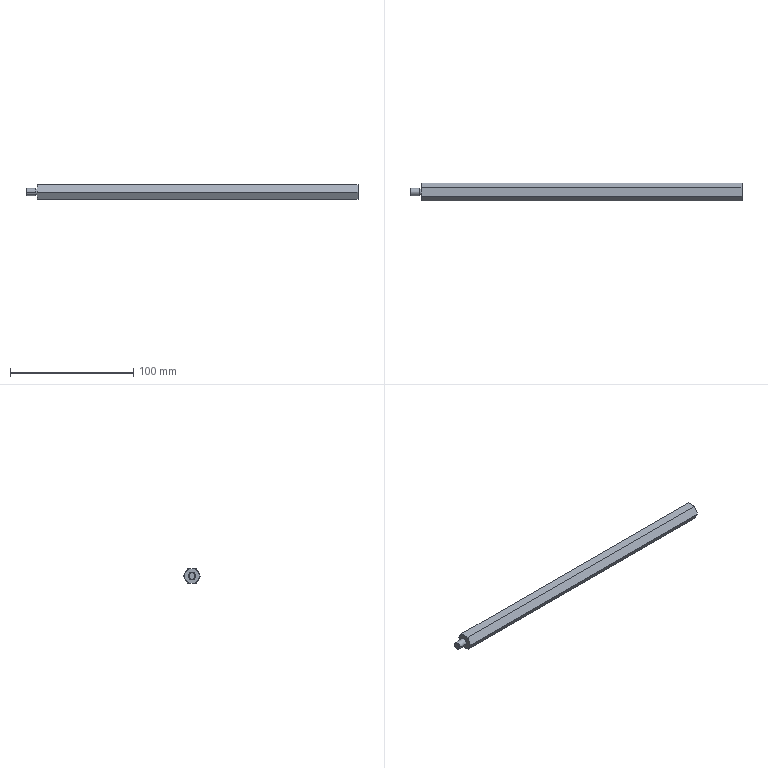Part | NX | 1 solid | 31 faces | box 269 x 13.856 x 12 mm | volume 32453 mm3 | cone 13 | plane 10 | cylinder 8 | commonest cylinder face diameters 4.2 x4 4.917 x2 6 x2
STEP:
#1=CARTESIAN_POINT('',(0.,5.196,-3.));
#2=VERTEX_POINT('',#1);
#3=CARTESIAN_POINT('',(0.5359,6.928,0.));
#4=VERTEX_POINT('',#3);
#5=CARTESIAN_POINT('',(0.,5.196,-3.));
#6=CARTESIAN_POINT('',(0.,5.754,-2.033));
#7=CARTESIAN_POINT('',(0.1777,6.308,-1.074));
#8=CARTESIAN_POINT('',(0.5359,6.928,0.));
#9=B_SPLINE_CURVE_WITH_KNOTS('',3,(#5,#6,#7,#8),.UNSPECIFIED.,.F.,.F.,(4,4),(0.,1.),.UNSPECIFIED.);
#10=EDGE_CURVE('',#2,#4,#9,.T.);
#11=ORIENTED_EDGE('',*,*,#10,.F.);
#12=CARTESIAN_POINT('',(0.,5.196,3.));
#13=VERTEX_POINT('',#12);
#14=CARTESIAN_POINT('',(0.,0.,0.));
#15=DIRECTION('',(1.,0.,0.));
#16=DIRECTION('',(0.,0.866,-0.5));
#17=AXIS2_PLACEMENT_3D('',#14,#15,#16);
#18=CIRCLE('',#17,6.);
#19=EDGE_CURVE('',#2,#13,#18,.T.);
#20=ORIENTED_EDGE('',*,*,#19,.T.);
#21=CARTESIAN_POINT('',(0.5359,6.928,0.));
#22=CARTESIAN_POINT('',(0.1786,6.309,1.072));
#23=CARTESIAN_POINT('',(0.,5.732,2.072));
#24=CARTESIAN_POINT('',(0.,5.196,3.));
#25=B_SPLINE_CURVE_WITH_KNOTS('',3,(#21,#22,#23,#24),.UNSPECIFIED.,.F.,.F.,(4,4),(0.,1.),.UNSPECIFIED.);
#26=EDGE_CURVE('',#13,#4,#25,.F.);
#27=ORIENTED_EDGE('',*,*,#26,.T.);
#28=EDGE_LOOP('',(#11,#20,#27));
#29=FACE_BOUND('',#28,.T.);
#30=CARTESIAN_POINT('',(0.2679,0.,0.));
#31=DIRECTION('',(1.,0.,0.));
#32=DIRECTION('',(0.,-1.,0.));
#33=AXIS2_PLACEMENT_3D('',#30,#31,#32);
#34=CONICAL_SURFACE('',#33,6.464,1.047);
#35=ADVANCED_FACE('',(#29),#34,.T.);
#36=CARTESIAN_POINT('',(-8.459,-3.,0.));
#37=VERTEX_POINT('',#36);
#38=CARTESIAN_POINT('',(-8.459,3.,0.));
#39=VERTEX_POINT('',#38);
#40=CARTESIAN_POINT('',(-8.459,0.,0.));
#41=DIRECTION('',(1.,0.,0.));
#42=DIRECTION('',(0.,1.,0.));
#43=AXIS2_PLACEMENT_3D('',#40,#41,#42);
#44=CIRCLE('',#43,3.);
#45=EDGE_CURVE('',#37,#39,#44,.T.);
#46=ORIENTED_EDGE('',*,*,#45,.F.);
#47=CARTESIAN_POINT('',(-9.,-2.459,0.));
#48=VERTEX_POINT('',#47);
#49=CARTESIAN_POINT('',(-8.729,-2.729,0.));
#50=DIRECTION('',(0.7071,-0.7071,0.));
#51=VECTOR('',#50,1000.);
#52=LINE('',#49,#51);
#53=EDGE_CURVE('',#37,#48,#52,.F.);
#54=ORIENTED_EDGE('',*,*,#53,.T.);
#55=CARTESIAN_POINT('',(-9.,2.459,0.));
#56=VERTEX_POINT('',#55);
#57=CARTESIAN_POINT('',(-9.,0.,0.));
#58=DIRECTION('',(1.,0.,0.));
#59=DIRECTION('',(0.,1.,0.));
#60=AXIS2_PLACEMENT_3D('',#57,#58,#59);
#61=CIRCLE('',#60,2.458);
#62=EDGE_CURVE('',#48,#56,#61,.T.);
#63=ORIENTED_EDGE('',*,*,#62,.T.);
#64=CARTESIAN_POINT('',(-8.729,2.729,0.));
#65=DIRECTION('',(0.7071,0.7071,0.));
#66=VECTOR('',#65,1000.);
#67=LINE('',#64,#66);
#68=EDGE_CURVE('',#39,#56,#67,.F.);
#69=ORIENTED_EDGE('',*,*,#68,.F.);
#70=EDGE_LOOP('',(#46,#54,#63,#69));
#71=FACE_BOUND('',#70,.T.);
#72=CARTESIAN_POINT('',(-8.729,0.,0.));
#73=DIRECTION('',(1.,0.,0.));
#74=DIRECTION('',(0.,-1.,0.));
#75=AXIS2_PLACEMENT_3D('',#72,#73,#74);
#76=CONICAL_SURFACE('',#75,2.729,0.7854);
#77=ADVANCED_FACE('',(#71),#76,.T.);
#78=CARTESIAN_POINT('',(260.,3.464,6.));
#79=VERTEX_POINT('',#78);
#80=CARTESIAN_POINT('',(260.,6.928,0.));
#81=VERTEX_POINT('',#80);
#82=CARTESIAN_POINT('',(260.,6.928,0.));
#83=DIRECTION('',(0.,0.5,-0.866));
#84=VECTOR('',#83,1000.);
#85=LINE('',#82,#84);
#86=EDGE_CURVE('',#79,#81,#85,.T.);
#87=ORIENTED_EDGE('',*,*,#86,.T.);
#88=CARTESIAN_POINT('',(260.,6.928,0.));
#89=DIRECTION('',(-1.,0.,0.));
#90=VECTOR('',#89,1000.);
#91=LINE('',#88,#90);
#92=EDGE_CURVE('',#81,#4,#91,.T.);
#93=ORIENTED_EDGE('',*,*,#92,.T.);
#94=ORIENTED_EDGE('',*,*,#26,.F.);
#95=CARTESIAN_POINT('',(0.5359,3.464,6.));
#96=VERTEX_POINT('',#95);
#97=CARTESIAN_POINT('',(0.,5.196,3.));
#98=CARTESIAN_POINT('',(0.,4.66,3.928));
#99=CARTESIAN_POINT('',(0.1786,4.083,4.928));
#100=CARTESIAN_POINT('',(0.5359,3.464,6.));
#101=B_SPLINE_CURVE_WITH_KNOTS('',3,(#97,#98,#99,#100),.UNSPECIFIED.,.F.,.F.,(4,4),(0.,1.),.UNSPECIFIED.);
#102=EDGE_CURVE('',#96,#13,#101,.F.);
#103=ORIENTED_EDGE('',*,*,#102,.F.);
#104=CARTESIAN_POINT('',(0.5359,3.464,6.));
#105=DIRECTION('',(1.,0.,0.));
#106=VECTOR('',#105,1000.);
#107=LINE('',#104,#106);
#108=EDGE_CURVE('',#96,#79,#107,.T.);
#109=ORIENTED_EDGE('',*,*,#108,.T.);
#110=EDGE_LOOP('',(#87,#93,#94,#103,#109));
#111=FACE_BOUND('',#110,.T.);
#112=CARTESIAN_POINT('',(155.,5.196,3.));
#113=DIRECTION('',(0.,-0.866,-0.5));
#114=DIRECTION('',(0.,0.5,-0.866));
#115=AXIS2_PLACEMENT_3D('',#112,#113,#114);
#116=PLANE('',#115);
#117=ADVANCED_FACE('',(#111),#116,.F.);
#118=CARTESIAN_POINT('',(260.,3.464,-6.));
#119=VERTEX_POINT('',#118);
#120=CARTESIAN_POINT('',(260.,-3.464,-6.));
#121=VERTEX_POINT('',#120);
#122=CARTESIAN_POINT('',(260.,0.,-6.));
#123=DIRECTION('',(0.,-1.,0.));
#124=VECTOR('',#123,1000.);
#125=LINE('',#122,#124);
#126=EDGE_CURVE('',#119,#121,#125,.T.);
#127=ORIENTED_EDGE('',*,*,#126,.F.);
#128=CARTESIAN_POINT('',(260.,6.928,0.));
#129=DIRECTION('',(0.,-0.5,-0.866));
#130=VECTOR('',#129,1000.);
#131=LINE('',#128,#130);
#132=EDGE_CURVE('',#81,#119,#131,.T.);
#133=ORIENTED_EDGE('',*,*,#132,.F.);
#134=ORIENTED_EDGE('',*,*,#86,.F.);
#135=CARTESIAN_POINT('',(260.,-3.464,6.));
#136=VERTEX_POINT('',#135);
#137=CARTESIAN_POINT('',(260.,0.,6.));
#138=DIRECTION('',(0.,1.,0.));
#139=VECTOR('',#138,1000.);
#140=LINE('',#137,#139);
#141=EDGE_CURVE('',#136,#79,#140,.T.);
#142=ORIENTED_EDGE('',*,*,#141,.F.);
#143=CARTESIAN_POINT('',(260.,-6.928,0.));
#144=VERTEX_POINT('',#143);
#145=CARTESIAN_POINT('',(260.,-6.928,0.));
#146=DIRECTION('',(0.,0.5,0.866));
#147=VECTOR('',#146,1000.);
#148=LINE('',#145,#147);
#149=EDGE_CURVE('',#144,#136,#148,.T.);
#150=ORIENTED_EDGE('',*,*,#149,.F.);
#151=CARTESIAN_POINT('',(260.,-6.928,0.));
#152=DIRECTION('',(0.,-0.5,0.866));
#153=VECTOR('',#152,1000.);
#154=LINE('',#151,#153);
#155=EDGE_CURVE('',#121,#144,#154,.T.);
#156=ORIENTED_EDGE('',*,*,#155,.F.);
#157=EDGE_LOOP('',(#127,#133,#134,#142,#150,#156));
#158=FACE_BOUND('',#157,.T.);
#159=CARTESIAN_POINT('',(260.,2.86,0.));
#160=VERTEX_POINT('',#159);
#161=CARTESIAN_POINT('',(260.,-2.86,0.));
#162=VERTEX_POINT('',#161);
#163=CARTESIAN_POINT('',(260.,0.,0.));
#164=DIRECTION('',(1.,0.,0.));
#165=DIRECTION('',(0.,-1.,0.));
#166=AXIS2_PLACEMENT_3D('',#163,#164,#165);
#167=CIRCLE('',#166,2.86);
#168=EDGE_CURVE('',#160,#162,#167,.T.);
#169=ORIENTED_EDGE('',*,*,#168,.F.);
#170=CARTESIAN_POINT('',(260.,0.,0.));
#171=DIRECTION('',(1.,0.,0.));
#172=DIRECTION('',(0.,-1.,0.));
#173=AXIS2_PLACEMENT_3D('',#170,#171,#172);
#174=CIRCLE('',#173,2.86);
#175=EDGE_CURVE('',#162,#160,#174,.T.);
#176=ORIENTED_EDGE('',*,*,#175,.F.);
#177=EDGE_LOOP('',(#169,#176));
#178=FACE_BOUND('',#177,.T.);
#179=CARTESIAN_POINT('',(260.,-6.371,11.678));
#180=DIRECTION('',(-1.,0.,0.));
#181=DIRECTION('',(0.,0.,1.));
#182=AXIS2_PLACEMENT_3D('',#179,#180,#181);
#183=PLANE('',#182);
#184=ADVANCED_FACE('',(#158,#178),#183,.F.);
#185=ORIENTED_EDGE('',*,*,#126,.T.);
#186=CARTESIAN_POINT('',(0.5359,-3.464,-6.));
#187=VERTEX_POINT('',#186);
#188=CARTESIAN_POINT('',(260.,-3.464,-6.));
#189=DIRECTION('',(-1.,0.,0.));
#190=VECTOR('',#189,1000.);
#191=LINE('',#188,#190);
#192=EDGE_CURVE('',#121,#187,#191,.T.);
#193=ORIENTED_EDGE('',*,*,#192,.T.);
#194=CARTESIAN_POINT('',(0.,0.,-6.));
#195=VERTEX_POINT('',#194);
#196=CARTESIAN_POINT('',(0.5359,-3.464,-6.));
#197=CARTESIAN_POINT('',(0.1786,-2.226,-6.));
#198=CARTESIAN_POINT('',(0.,-1.072,-6.));
#199=CARTESIAN_POINT('',(0.,0.,-6.));
#200=B_SPLINE_CURVE_WITH_KNOTS('',3,(#196,#197,#198,#199),.UNSPECIFIED.,.F.,.F.,(4,4),(0.,1.),.UNSPECIFIED.);
#201=EDGE_CURVE('',#195,#187,#200,.F.);
#202=ORIENTED_EDGE('',*,*,#201,.F.);
#203=CARTESIAN_POINT('',(0.5359,3.464,-6.));
#204=VERTEX_POINT('',#203);
#205=CARTESIAN_POINT('',(0.,0.,-6.));
#206=CARTESIAN_POINT('',(0.,1.072,-6.));
#207=CARTESIAN_POINT('',(0.1786,2.226,-6.));
#208=CARTESIAN_POINT('',(0.5359,3.464,-6.));
#209=B_SPLINE_CURVE_WITH_KNOTS('',3,(#205,#206,#207,#208),.UNSPECIFIED.,.F.,.F.,(4,4),(0.,1.),.UNSPECIFIED.);
#210=EDGE_CURVE('',#204,#195,#209,.F.);
#211=ORIENTED_EDGE('',*,*,#210,.F.);
#212=CARTESIAN_POINT('',(0.5359,3.464,-6.));
#213=DIRECTION('',(1.,0.,0.));
#214=VECTOR('',#213,1000.);
#215=LINE('',#212,#214);
#216=EDGE_CURVE('',#204,#119,#215,.T.);
#217=ORIENTED_EDGE('',*,*,#216,.T.);
#218=EDGE_LOOP('',(#185,#193,#202,#211,#217));
#219=FACE_BOUND('',#218,.T.);
#220=CARTESIAN_POINT('',(155.,0.,-6.));
#221=DIRECTION('',(0.,0.,1.));
#222=DIRECTION('',(1.,0.,0.));
#223=AXIS2_PLACEMENT_3D('',#220,#221,#222);
#224=PLANE('',#223);
#225=ADVANCED_FACE('',(#219),#224,.F.);
#226=ORIENTED_EDGE('',*,*,#132,.T.);
#227=ORIENTED_EDGE('',*,*,#216,.F.);
#228=CARTESIAN_POINT('',(0.5359,3.464,-6.));
#229=CARTESIAN_POINT('',(0.1786,4.083,-4.928));
#230=CARTESIAN_POINT('',(0.,4.66,-3.928));
#231=CARTESIAN_POINT('',(0.,5.196,-3.));
#232=B_SPLINE_CURVE_WITH_KNOTS('',3,(#228,#229,#230,#231),.UNSPECIFIED.,.F.,.F.,(4,4),(0.,1.),.UNSPECIFIED.);
#233=EDGE_CURVE('',#2,#204,#232,.F.);
#234=ORIENTED_EDGE('',*,*,#233,.F.);
#235=ORIENTED_EDGE('',*,*,#10,.T.);
#236=ORIENTED_EDGE('',*,*,#92,.F.);
#237=EDGE_LOOP('',(#226,#227,#234,#235,#236));
#238=FACE_BOUND('',#237,.T.);
#239=CARTESIAN_POINT('',(155.,5.196,-3.));
#240=DIRECTION('',(0.,-0.866,0.5));
#241=DIRECTION('',(-1.,0.,0.));
#242=AXIS2_PLACEMENT_3D('',#239,#240,#241);
#243=PLANE('',#242);
#244=ADVANCED_FACE('',(#238),#243,.F.);
#245=ORIENTED_EDGE('',*,*,#210,.T.);
#246=CARTESIAN_POINT('',(0.,0.,0.));
#247=DIRECTION('',(1.,0.,0.));
#248=DIRECTION('',(0.,0.,-1.));
#249=AXIS2_PLACEMENT_3D('',#246,#247,#248);
#250=CIRCLE('',#249,6.);
#251=EDGE_CURVE('',#195,#2,#250,.T.);
#252=ORIENTED_EDGE('',*,*,#251,.T.);
#253=ORIENTED_EDGE('',*,*,#233,.T.);
#254=EDGE_LOOP('',(#245,#252,#253));
#255=FACE_BOUND('',#254,.T.);
#256=CARTESIAN_POINT('',(0.2679,0.,0.));
#257=DIRECTION('',(1.,0.,0.));
#258=DIRECTION('',(0.,-1.,0.));
#259=AXIS2_PLACEMENT_3D('',#256,#257,#258);
#260=CONICAL_SURFACE('',#259,6.464,1.047);
#261=ADVANCED_FACE('',(#255),#260,.T.);
#262=ORIENTED_EDGE('',*,*,#19,.F.);
#263=ORIENTED_EDGE('',*,*,#251,.F.);
#264=CARTESIAN_POINT('',(0.,-5.196,-3.));
#265=VERTEX_POINT('',#264);
#266=CARTESIAN_POINT('',(0.,0.,0.));
#267=DIRECTION('',(1.,0.,0.));
#268=DIRECTION('',(0.,-0.866,-0.5));
#269=AXIS2_PLACEMENT_3D('',#266,#267,#268);
#270=CIRCLE('',#269,6.);
#271=EDGE_CURVE('',#265,#195,#270,.T.);
#272=ORIENTED_EDGE('',*,*,#271,.F.);
#273=CARTESIAN_POINT('',(0.,-6.,0.));
#274=VERTEX_POINT('',#273);
#275=CARTESIAN_POINT('',(0.,0.,0.));
#276=DIRECTION('',(1.,0.,0.));
#277=DIRECTION('',(0.,-1.,0.));
#278=AXIS2_PLACEMENT_3D('',#275,#276,#277);
#279=CIRCLE('',#278,6.);
#280=EDGE_CURVE('',#274,#265,#279,.T.);
#281=ORIENTED_EDGE('',*,*,#280,.F.);
#282=CARTESIAN_POINT('',(0.,-5.196,3.));
#283=VERTEX_POINT('',#282);
#284=CARTESIAN_POINT('',(0.,0.,0.));
#285=DIRECTION('',(1.,0.,0.));
#286=DIRECTION('',(0.,-1.,0.));
#287=AXIS2_PLACEMENT_3D('',#284,#285,#286);
#288=CIRCLE('',#287,6.);
#289=EDGE_CURVE('',#283,#274,#288,.T.);
#290=ORIENTED_EDGE('',*,*,#289,.F.);
#291=CARTESIAN_POINT('',(0.,0.,6.));
#292=VERTEX_POINT('',#291);
#293=CARTESIAN_POINT('',(0.,0.,0.));
#294=DIRECTION('',(1.,0.,0.));
#295=DIRECTION('',(0.,0.,1.));
#296=AXIS2_PLACEMENT_3D('',#293,#294,#295);
#297=CIRCLE('',#296,6.);
#298=EDGE_CURVE('',#292,#283,#297,.T.);
#299=ORIENTED_EDGE('',*,*,#298,.F.);
#300=CARTESIAN_POINT('',(0.,0.,0.));
#301=DIRECTION('',(1.,0.,0.));
#302=DIRECTION('',(0.,0.866,0.5));
#303=AXIS2_PLACEMENT_3D('',#300,#301,#302);
#304=CIRCLE('',#303,6.);
#305=EDGE_CURVE('',#13,#292,#304,.T.);
#306=ORIENTED_EDGE('',*,*,#305,.F.);
#307=EDGE_LOOP('',(#262,#263,#272,#281,#290,#299,#306));
#308=FACE_BOUND('',#307,.T.);
#309=CARTESIAN_POINT('',(0.,-2.458,0.));
#310=VERTEX_POINT('',#309);
#311=CARTESIAN_POINT('',(0.,2.458,0.));
#312=VERTEX_POINT('',#311);
#313=CARTESIAN_POINT('',(0.,0.,0.));
#314=DIRECTION('',(-1.,0.,0.));
#315=DIRECTION('',(0.,1.,0.));
#316=AXIS2_PLACEMENT_3D('',#313,#314,#315);
#317=CIRCLE('',#316,2.458);
#318=EDGE_CURVE('',#310,#312,#317,.T.);
#319=ORIENTED_EDGE('',*,*,#318,.F.);
#320=CARTESIAN_POINT('',(0.,0.,0.));
#321=DIRECTION('',(-1.,0.,0.));
#322=DIRECTION('',(0.,1.,0.));
#323=AXIS2_PLACEMENT_3D('',#320,#321,#322);
#324=CIRCLE('',#323,2.458);
#325=EDGE_CURVE('',#312,#310,#324,.T.);
#326=ORIENTED_EDGE('',*,*,#325,.F.);
#327=EDGE_LOOP('',(#319,#326));
#328=FACE_BOUND('',#327,.T.);
#329=CARTESIAN_POINT('',(0.,0.,0.));
#330=DIRECTION('',(1.,0.,0.));
#331=DIRECTION('',(0.,1.,0.));
#332=AXIS2_PLACEMENT_3D('',#329,#330,#331);
#333=PLANE('',#332);
#334=ADVANCED_FACE('',(#308,#328),#333,.F.);
#335=CARTESIAN_POINT('',(0.5359,3.464,6.));
#336=CARTESIAN_POINT('',(0.1786,2.226,6.));
#337=CARTESIAN_POINT('',(0.,1.072,6.));
#338=CARTESIAN_POINT('',(0.,0.,6.));
#339=B_SPLINE_CURVE_WITH_KNOTS('',3,(#335,#336,#337,#338),.UNSPECIFIED.,.F.,.F.,(4,4),(0.,1.),.UNSPECIFIED.);
#340=EDGE_CURVE('',#292,#96,#339,.F.);
#341=ORIENTED_EDGE('',*,*,#340,.T.);
#342=ORIENTED_EDGE('',*,*,#102,.T.);
#343=ORIENTED_EDGE('',*,*,#305,.T.);
#344=EDGE_LOOP('',(#341,#342,#343));
#345=FACE_BOUND('',#344,.T.);
#346=CARTESIAN_POINT('',(0.2679,0.,0.));
#347=DIRECTION('',(1.,0.,0.));
#348=DIRECTION('',(0.,-1.,0.));
#349=AXIS2_PLACEMENT_3D('',#346,#347,#348);
#350=CONICAL_SURFACE('',#349,6.464,1.047);
#351=ADVANCED_FACE('',(#345),#350,.T.);
#352=ORIENTED_EDGE('',*,*,#141,.T.);
#353=ORIENTED_EDGE('',*,*,#108,.F.);
#354=ORIENTED_EDGE('',*,*,#340,.F.);
#355=CARTESIAN_POINT('',(0.5359,-3.464,6.));
#356=VERTEX_POINT('',#355);
#357=CARTESIAN_POINT('',(0.,0.,6.));
#358=CARTESIAN_POINT('',(0.,-1.072,6.));
#359=CARTESIAN_POINT('',(0.1786,-2.226,6.));
#360=CARTESIAN_POINT('',(0.5359,-3.464,6.));
#361=B_SPLINE_CURVE_WITH_KNOTS('',3,(#357,#358,#359,#360),.UNSPECIFIED.,.F.,.F.,(4,4),(0.,1.),.UNSPECIFIED.);
#362=EDGE_CURVE('',#356,#292,#361,.F.);
#363=ORIENTED_EDGE('',*,*,#362,.F.);
#364=CARTESIAN_POINT('',(0.5359,-3.464,6.));
#365=DIRECTION('',(1.,0.,0.));
#366=VECTOR('',#365,1000.);
#367=LINE('',#364,#366);
#368=EDGE_CURVE('',#356,#136,#367,.T.);
#369=ORIENTED_EDGE('',*,*,#368,.T.);
#370=EDGE_LOOP('',(#352,#353,#354,#363,#369));
#371=FACE_BOUND('',#370,.T.);
#372=CARTESIAN_POINT('',(155.,0.,6.));
#373=DIRECTION('',(0.,0.,-1.));
#374=DIRECTION('',(0.,-1.,0.));
#375=AXIS2_PLACEMENT_3D('',#372,#373,#374);
#376=PLANE('',#375);
#377=ADVANCED_FACE('',(#371),#376,.F.);
#378=ORIENTED_EDGE('',*,*,#149,.T.);
#379=ORIENTED_EDGE('',*,*,#368,.F.);
#380=CARTESIAN_POINT('',(0.5359,-3.464,6.));
#381=CARTESIAN_POINT('',(0.1786,-4.083,4.928));
#382=CARTESIAN_POINT('',(0.,-4.66,3.928));
#383=CARTESIAN_POINT('',(0.,-5.196,3.));
#384=B_SPLINE_CURVE_WITH_KNOTS('',3,(#380,#381,#382,#383),.UNSPECIFIED.,.F.,.F.,(4,4),(0.,1.),.UNSPECIFIED.);
#385=EDGE_CURVE('',#283,#356,#384,.F.);
#386=ORIENTED_EDGE('',*,*,#385,.F.);
#387=CARTESIAN_POINT('',(0.5359,-6.928,0.));
#388=VERTEX_POINT('',#387);
#389=CARTESIAN_POINT('',(0.,-5.196,3.));
#390=CARTESIAN_POINT('',(0.,-5.732,2.072));
#391=CARTESIAN_POINT('',(0.1786,-6.309,1.072));
#392=CARTESIAN_POINT('',(0.5359,-6.928,0.));
#393=B_SPLINE_CURVE_WITH_KNOTS('',3,(#389,#390,#391,#392),.UNSPECIFIED.,.F.,.F.,(4,4),(0.,1.),.UNSPECIFIED.);
#394=EDGE_CURVE('',#388,#283,#393,.F.);
#395=ORIENTED_EDGE('',*,*,#394,.F.);
#396=CARTESIAN_POINT('',(0.5359,-6.928,0.));
#397=DIRECTION('',(1.,0.,0.));
#398=VECTOR('',#397,1000.);
#399=LINE('',#396,#398);
#400=EDGE_CURVE('',#388,#144,#399,.T.);
#401=ORIENTED_EDGE('',*,*,#400,.T.);
#402=EDGE_LOOP('',(#378,#379,#386,#395,#401));
#403=FACE_BOUND('',#402,.T.);
#404=CARTESIAN_POINT('',(155.,-5.196,3.));
#405=DIRECTION('',(0.,0.866,-0.5));
#406=DIRECTION('',(-1.,0.,0.));
#407=AXIS2_PLACEMENT_3D('',#404,#405,#406);
#408=PLANE('',#407);
#409=ADVANCED_FACE('',(#403),#408,.F.);
#410=ORIENTED_EDGE('',*,*,#155,.T.);
#411=ORIENTED_EDGE('',*,*,#400,.F.);
#412=CARTESIAN_POINT('',(0.5359,-6.928,0.));
#413=CARTESIAN_POINT('',(0.1781,-6.308,-1.073));
#414=CARTESIAN_POINT('',(0.,-5.755,-2.032));
#415=CARTESIAN_POINT('',(0.,-5.196,-3.));
#416=B_SPLINE_CURVE_WITH_KNOTS('',3,(#412,#413,#414,#415),.UNSPECIFIED.,.F.,.F.,(4,4),(0.,1.),.UNSPECIFIED.);
#417=EDGE_CURVE('',#388,#265,#416,.T.);
#418=ORIENTED_EDGE('',*,*,#417,.T.);
#419=CARTESIAN_POINT('',(0.,-5.196,-3.));
#420=CARTESIAN_POINT('',(0.,-4.66,-3.928));
#421=CARTESIAN_POINT('',(0.1786,-4.083,-4.928));
#422=CARTESIAN_POINT('',(0.5359,-3.464,-6.));
#423=B_SPLINE_CURVE_WITH_KNOTS('',3,(#419,#420,#421,#422),.UNSPECIFIED.,.F.,.F.,(4,4),(0.,1.),.UNSPECIFIED.);
#424=EDGE_CURVE('',#187,#265,#423,.F.);
#425=ORIENTED_EDGE('',*,*,#424,.F.);
#426=ORIENTED_EDGE('',*,*,#192,.F.);
#427=EDGE_LOOP('',(#410,#411,#418,#425,#426));
#428=FACE_BOUND('',#427,.T.);
#429=CARTESIAN_POINT('',(155.,-5.196,-3.));
#430=DIRECTION('',(0.,0.866,0.5));
#431=DIRECTION('',(1.,0.,0.));
#432=AXIS2_PLACEMENT_3D('',#429,#430,#431);
#433=PLANE('',#432);
#434=ADVANCED_FACE('',(#428),#433,.F.);
#435=ORIENTED_EDGE('',*,*,#424,.T.);
#436=ORIENTED_EDGE('',*,*,#271,.T.);
#437=ORIENTED_EDGE('',*,*,#201,.T.);
#438=EDGE_LOOP('',(#435,#436,#437));
#439=FACE_BOUND('',#438,.T.);
#440=CARTESIAN_POINT('',(0.2679,0.,0.));
#441=DIRECTION('',(1.,0.,0.));
#442=DIRECTION('',(0.,-1.,0.));
#443=AXIS2_PLACEMENT_3D('',#440,#441,#442);
#444=CONICAL_SURFACE('',#443,6.464,1.047);
#445=ADVANCED_FACE('',(#439),#444,.T.);
#446=CARTESIAN_POINT('',(0.2679,-6.464,0.));
#447=DIRECTION('',(0.5,-0.866,0.));
#448=VECTOR('',#447,1000.);
#449=LINE('',#446,#448);
#450=EDGE_CURVE('',#274,#388,#449,.T.);
#451=ORIENTED_EDGE('',*,*,#450,.F.);
#452=ORIENTED_EDGE('',*,*,#280,.T.);
#453=ORIENTED_EDGE('',*,*,#417,.F.);
#454=EDGE_LOOP('',(#451,#452,#453));
#455=FACE_BOUND('',#454,.T.);
#456=CARTESIAN_POINT('',(0.2679,0.,0.));
#457=DIRECTION('',(1.,0.,0.));
#458=DIRECTION('',(0.,-1.,0.));
#459=AXIS2_PLACEMENT_3D('',#456,#457,#458);
#460=CONICAL_SURFACE('',#459,6.464,1.047);
#461=ADVANCED_FACE('',(#455),#460,.T.);
#462=ORIENTED_EDGE('',*,*,#45,.T.);
#463=CARTESIAN_POINT('',(-0.9,3.,0.));
#464=VERTEX_POINT('',#463);
#465=CARTESIAN_POINT('',(-8.459,3.,0.));
#466=DIRECTION('',(-1.,0.,0.));
#467=VECTOR('',#466,1000.);
#468=LINE('',#465,#467);
#469=EDGE_CURVE('',#464,#39,#468,.T.);
#470=ORIENTED_EDGE('',*,*,#469,.F.);
#471=CARTESIAN_POINT('',(-0.9,-3.,0.));
#472=VERTEX_POINT('',#471);
#473=CARTESIAN_POINT('',(-0.9,0.,0.));
#474=DIRECTION('',(-1.,0.,0.));
#475=DIRECTION('',(0.,-1.,0.));
#476=AXIS2_PLACEMENT_3D('',#473,#474,#475);
#477=CIRCLE('',#476,3.);
#478=EDGE_CURVE('',#464,#472,#477,.T.);
#479=ORIENTED_EDGE('',*,*,#478,.T.);
#480=CARTESIAN_POINT('',(-8.459,-3.,0.));
#481=DIRECTION('',(-1.,0.,0.));
#482=VECTOR('',#481,1000.);
#483=LINE('',#480,#482);
#484=EDGE_CURVE('',#472,#37,#483,.T.);
#485=ORIENTED_EDGE('',*,*,#484,.T.);
#486=EDGE_LOOP('',(#462,#470,#479,#485));
#487=FACE_BOUND('',#486,.T.);
#488=CARTESIAN_POINT('',(-8.459,0.,0.));
#489=DIRECTION('',(-1.,0.,0.));
#490=DIRECTION('',(0.,1.,0.));
#491=AXIS2_PLACEMENT_3D('',#488,#489,#490);
#492=CYLINDRICAL_SURFACE('',#491,3.);
#493=ADVANCED_FACE('',(#487),#492,.T.);
#494=ORIENTED_EDGE('',*,*,#385,.T.);
#495=ORIENTED_EDGE('',*,*,#362,.T.);
#496=ORIENTED_EDGE('',*,*,#298,.T.);
#497=EDGE_LOOP('',(#494,#495,#496));
#498=FACE_BOUND('',#497,.T.);
#499=CARTESIAN_POINT('',(0.2679,0.,0.));
#500=DIRECTION('',(1.,0.,0.));
#501=DIRECTION('',(0.,-1.,0.));
#502=AXIS2_PLACEMENT_3D('',#499,#500,#501);
#503=CONICAL_SURFACE('',#502,6.464,1.047);
#504=ADVANCED_FACE('',(#498),#503,.T.);
#505=ORIENTED_EDGE('',*,*,#318,.T.);
#506=CARTESIAN_POINT('',(-0.9,2.458,0.));
#507=VERTEX_POINT('',#506);
#508=CARTESIAN_POINT('',(-0.9,2.458,0.));
#509=DIRECTION('',(-1.,0.,0.));
#510=VECTOR('',#509,1000.);
#511=LINE('',#508,#510);
#512=EDGE_CURVE('',#312,#507,#511,.T.);
#513=ORIENTED_EDGE('',*,*,#512,.T.);
#514=CARTESIAN_POINT('',(-0.9,-2.458,0.));
#515=VERTEX_POINT('',#514);
#516=CARTESIAN_POINT('',(-0.9,0.,0.));
#517=DIRECTION('',(1.,0.,0.));
#518=DIRECTION('',(0.,1.,0.));
#519=AXIS2_PLACEMENT_3D('',#516,#517,#518);
#520=CIRCLE('',#519,2.458);
#521=EDGE_CURVE('',#507,#515,#520,.T.);
#522=ORIENTED_EDGE('',*,*,#521,.T.);
#523=CARTESIAN_POINT('',(-0.9,-2.458,0.));
#524=DIRECTION('',(-1.,0.,0.));
#525=VECTOR('',#524,1000.);
#526=LINE('',#523,#525);
#527=EDGE_CURVE('',#310,#515,#526,.T.);
#528=ORIENTED_EDGE('',*,*,#527,.F.);
#529=EDGE_LOOP('',(#505,#513,#522,#528));
#530=FACE_BOUND('',#529,.T.);
#531=CARTESIAN_POINT('',(-0.9,0.,0.));
#532=DIRECTION('',(-1.,0.,0.));
#533=DIRECTION('',(0.,1.,0.));
#534=AXIS2_PLACEMENT_3D('',#531,#532,#533);
#535=CYLINDRICAL_SURFACE('',#534,2.458);
#536=ADVANCED_FACE('',(#530),#535,.T.);
#537=ORIENTED_EDGE('',*,*,#62,.F.);
#538=CARTESIAN_POINT('',(-9.,0.,0.));
#539=DIRECTION('',(1.,0.,0.));
#540=DIRECTION('',(0.,1.,0.));
#541=AXIS2_PLACEMENT_3D('',#538,#539,#540);
#542=CIRCLE('',#541,2.458);
#543=EDGE_CURVE('',#56,#48,#542,.T.);
#544=ORIENTED_EDGE('',*,*,#543,.F.);
#545=EDGE_LOOP('',(#537,#544));
#546=FACE_BOUND('',#545,.T.);
#547=CARTESIAN_POINT('',(-9.,0.,0.));
#548=DIRECTION('',(1.,0.,0.));
#549=DIRECTION('',(0.,1.,0.));
#550=AXIS2_PLACEMENT_3D('',#547,#548,#549);
#551=PLANE('',#550);
#552=ADVANCED_FACE('',(#546),#551,.F.);
#553=CARTESIAN_POINT('',(-0.9,0.,0.));
#554=DIRECTION('',(-1.,0.,0.));
#555=DIRECTION('',(0.,-1.,0.));
#556=AXIS2_PLACEMENT_3D('',#553,#554,#555);
#557=CIRCLE('',#556,3.);
#558=EDGE_CURVE('',#472,#464,#557,.T.);
#559=ORIENTED_EDGE('',*,*,#558,.F.);
#560=ORIENTED_EDGE('',*,*,#478,.F.);
#561=EDGE_LOOP('',(#559,#560));
#562=FACE_BOUND('',#561,.T.);
#563=CARTESIAN_POINT('',(-0.9,0.,0.));
#564=DIRECTION('',(1.,0.,0.));
#565=DIRECTION('',(0.,1.,0.));
#566=AXIS2_PLACEMENT_3D('',#563,#564,#565);
#567=CIRCLE('',#566,2.458);
#568=EDGE_CURVE('',#515,#507,#567,.T.);
#569=ORIENTED_EDGE('',*,*,#568,.F.);
#570=ORIENTED_EDGE('',*,*,#521,.F.);
#571=EDGE_LOOP('',(#569,#570));
#572=FACE_BOUND('',#571,.T.);
#573=CARTESIAN_POINT('',(-0.9,0.,0.));
#574=DIRECTION('',(-1.,0.,0.));
#575=DIRECTION('',(0.,0.,1.));
#576=AXIS2_PLACEMENT_3D('',#573,#574,#575);
#577=PLANE('',#576);
#578=ADVANCED_FACE('',(#562,#572),#577,.F.);
#579=CARTESIAN_POINT('',(259.561,2.1,0.));
#580=VERTEX_POINT('',#579);
#581=CARTESIAN_POINT('',(259.561,-2.1,0.));
#582=VERTEX_POINT('',#581);
#583=CARTESIAN_POINT('',(259.561,0.,0.));
#584=DIRECTION('',(1.,0.,0.));
#585=DIRECTION('',(0.,-1.,0.));
#586=AXIS2_PLACEMENT_3D('',#583,#584,#585);
#587=CIRCLE('',#586,2.1);
#588=EDGE_CURVE('',#580,#582,#587,.T.);
#589=ORIENTED_EDGE('',*,*,#588,.T.);
#590=CARTESIAN_POINT('',(248.,-2.1,0.));
#591=VERTEX_POINT('',#590);
#592=CARTESIAN_POINT('',(260.,-2.1,0.));
#593=DIRECTION('',(1.,0.,0.));
#594=VECTOR('',#593,1000.);
#595=LINE('',#592,#594);
#596=EDGE_CURVE('',#582,#591,#595,.F.);
#597=ORIENTED_EDGE('',*,*,#596,.T.);
#598=CARTESIAN_POINT('',(248.,2.1,0.));
#599=VERTEX_POINT('',#598);
#600=CARTESIAN_POINT('',(248.,0.,0.));
#601=DIRECTION('',(1.,0.,0.));
#602=DIRECTION('',(0.,-1.,0.));
#603=AXIS2_PLACEMENT_3D('',#600,#601,#602);
#604=CIRCLE('',#603,2.1);
#605=EDGE_CURVE('',#599,#591,#604,.T.);
#606=ORIENTED_EDGE('',*,*,#605,.F.);
#607=CARTESIAN_POINT('',(260.,2.1,0.));
#608=DIRECTION('',(1.,0.,0.));
#609=VECTOR('',#608,1000.);
#610=LINE('',#607,#609);
#611=EDGE_CURVE('',#580,#599,#610,.F.);
#612=ORIENTED_EDGE('',*,*,#611,.F.);
#613=EDGE_LOOP('',(#589,#597,#606,#612));
#614=FACE_BOUND('',#613,.T.);
#615=CARTESIAN_POINT('',(260.,0.,0.));
#616=DIRECTION('',(1.,0.,0.));
#617=DIRECTION('',(0.,-1.,0.));
#618=AXIS2_PLACEMENT_3D('',#615,#616,#617);
#619=CYLINDRICAL_SURFACE('',#618,2.1);
#620=ADVANCED_FACE('',(#614),#619,.F.);
#621=ORIENTED_EDGE('',*,*,#605,.T.);
#622=CARTESIAN_POINT('',(245.2,-2.1,0.));
#623=VERTEX_POINT('',#622);
#624=CARTESIAN_POINT('',(260.,-2.1,0.));
#625=DIRECTION('',(1.,0.,0.));
#626=VECTOR('',#625,1000.);
#627=LINE('',#624,#626);
#628=EDGE_CURVE('',#591,#623,#627,.F.);
#629=ORIENTED_EDGE('',*,*,#628,.T.);
#630=CARTESIAN_POINT('',(245.2,2.1,0.));
#631=VERTEX_POINT('',#630);
#632=CARTESIAN_POINT('',(245.2,0.,0.));
#633=DIRECTION('',(1.,0.,0.));
#634=DIRECTION('',(0.,-1.,0.));
#635=AXIS2_PLACEMENT_3D('',#632,#633,#634);
#636=CIRCLE('',#635,2.1);
#637=EDGE_CURVE('',#631,#623,#636,.T.);
#638=ORIENTED_EDGE('',*,*,#637,.F.);
#639=CARTESIAN_POINT('',(260.,2.1,0.));
#640=DIRECTION('',(1.,0.,0.));
#641=VECTOR('',#640,1000.);
#642=LINE('',#639,#641);
#643=EDGE_CURVE('',#599,#631,#642,.F.);
#644=ORIENTED_EDGE('',*,*,#643,.F.);
#645=EDGE_LOOP('',(#621,#629,#638,#644));
#646=FACE_BOUND('',#645,.T.);
#647=CARTESIAN_POINT('',(260.,0.,0.));
#648=DIRECTION('',(1.,0.,0.));
#649=DIRECTION('',(0.,-1.,0.));
#650=AXIS2_PLACEMENT_3D('',#647,#648,#649);
#651=CYLINDRICAL_SURFACE('',#650,2.1);
#652=ADVANCED_FACE('',(#646),#651,.F.);
#653=ORIENTED_EDGE('',*,*,#637,.T.);
#654=CARTESIAN_POINT('',(243.938,0.,0.));
#655=VERTEX_POINT('',#654);
#656=CARTESIAN_POINT('',(245.2,-2.1,0.));
#657=DIRECTION('',(0.515,-0.8572,0.));
#658=VECTOR('',#657,1000.);
#659=LINE('',#656,#658);
#660=EDGE_CURVE('',#655,#623,#659,.T.);
#661=ORIENTED_EDGE('',*,*,#660,.F.);
#662=CARTESIAN_POINT('',(245.2,2.1,0.));
#663=DIRECTION('',(0.515,0.8572,0.));
#664=VECTOR('',#663,1000.);
#665=LINE('',#662,#664);
#666=EDGE_CURVE('',#655,#631,#665,.T.);
#667=ORIENTED_EDGE('',*,*,#666,.T.);
#668=EDGE_LOOP('',(#653,#661,#667));
#669=FACE_BOUND('',#668,.T.);
#670=CARTESIAN_POINT('',(245.2,0.,0.));
#671=DIRECTION('',(1.,0.,0.));
#672=DIRECTION('',(0.,-1.,0.));
#673=AXIS2_PLACEMENT_3D('',#670,#671,#672);
#674=CONICAL_SURFACE('',#673,2.1,1.03);
#675=ADVANCED_FACE('',(#669),#674,.F.);
#676=ORIENTED_EDGE('',*,*,#588,.F.);
#677=CARTESIAN_POINT('',(259.561,2.1,0.));
#678=DIRECTION('',(0.5,0.866,0.));
#679=VECTOR('',#678,1000.);
#680=LINE('',#677,#679);
#681=EDGE_CURVE('',#160,#580,#680,.F.);
#682=ORIENTED_EDGE('',*,*,#681,.F.);
#683=ORIENTED_EDGE('',*,*,#168,.T.);
#684=CARTESIAN_POINT('',(259.561,-2.1,0.));
#685=DIRECTION('',(0.5,-0.866,0.));
#686=VECTOR('',#685,1000.);
#687=LINE('',#684,#686);
#688=EDGE_CURVE('',#162,#582,#687,.F.);
#689=ORIENTED_EDGE('',*,*,#688,.T.);
#690=EDGE_LOOP('',(#676,#682,#683,#689));
#691=FACE_BOUND('',#690,.T.);
#692=CARTESIAN_POINT('',(259.561,0.,0.));
#693=DIRECTION('',(1.,0.,0.));
#694=DIRECTION('',(0.,-1.,0.));
#695=AXIS2_PLACEMENT_3D('',#692,#693,#694);
#696=CONICAL_SURFACE('',#695,2.1,1.047);
#697=ADVANCED_FACE('',(#691),#696,.F.);
#698=ORIENTED_EDGE('',*,*,#568,.T.);
#699=ORIENTED_EDGE('',*,*,#512,.F.);
#700=ORIENTED_EDGE('',*,*,#325,.T.);
#701=ORIENTED_EDGE('',*,*,#527,.T.);
#702=EDGE_LOOP('',(#698,#699,#700,#701));
#703=FACE_BOUND('',#702,.T.);
#704=CARTESIAN_POINT('',(-0.9,0.,0.));
#705=DIRECTION('',(-1.,0.,0.));
#706=DIRECTION('',(0.,1.,0.));
#707=AXIS2_PLACEMENT_3D('',#704,#705,#706);
#708=CYLINDRICAL_SURFACE('',#707,2.458);
#709=ADVANCED_FACE('',(#703),#708,.T.);
#710=ORIENTED_EDGE('',*,*,#666,.F.);
#711=ORIENTED_EDGE('',*,*,#660,.T.);
#712=CARTESIAN_POINT('',(245.2,0.,0.));
#713=DIRECTION('',(1.,0.,0.));
#714=DIRECTION('',(0.,-1.,0.));
#715=AXIS2_PLACEMENT_3D('',#712,#713,#714);
#716=CIRCLE('',#715,2.1);
#717=EDGE_CURVE('',#623,#631,#716,.T.);
#718=ORIENTED_EDGE('',*,*,#717,.T.);
#719=EDGE_LOOP('',(#710,#711,#718));
#720=FACE_BOUND('',#719,.T.);
#721=CARTESIAN_POINT('',(245.2,0.,0.));
#722=DIRECTION('',(1.,0.,0.));
#723=DIRECTION('',(0.,-1.,0.));
#724=AXIS2_PLACEMENT_3D('',#721,#722,#723);
#725=CONICAL_SURFACE('',#724,2.1,1.03);
#726=ADVANCED_FACE('',(#720),#725,.F.);
#727=ORIENTED_EDGE('',*,*,#628,.F.);
#728=CARTESIAN_POINT('',(248.,0.,0.));
#729=DIRECTION('',(1.,0.,0.));
#730=DIRECTION('',(0.,-1.,0.));
#731=AXIS2_PLACEMENT_3D('',#728,#729,#730);
#732=CIRCLE('',#731,2.1);
#733=EDGE_CURVE('',#591,#599,#732,.T.);
#734=ORIENTED_EDGE('',*,*,#733,.T.);
#735=ORIENTED_EDGE('',*,*,#643,.T.);
#736=ORIENTED_EDGE('',*,*,#717,.F.);
#737=EDGE_LOOP('',(#727,#734,#735,#736));
#738=FACE_BOUND('',#737,.T.);
#739=CARTESIAN_POINT('',(260.,0.,0.));
#740=DIRECTION('',(1.,0.,0.));
#741=DIRECTION('',(0.,-1.,0.));
#742=AXIS2_PLACEMENT_3D('',#739,#740,#741);
#743=CYLINDRICAL_SURFACE('',#742,2.1);
#744=ADVANCED_FACE('',(#738),#743,.F.);
#745=ORIENTED_EDGE('',*,*,#596,.F.);
#746=CARTESIAN_POINT('',(259.561,0.,0.));
#747=DIRECTION('',(1.,0.,0.));
#748=DIRECTION('',(0.,-1.,0.));
#749=AXIS2_PLACEMENT_3D('',#746,#747,#748);
#750=CIRCLE('',#749,2.1);
#751=EDGE_CURVE('',#582,#580,#750,.T.);
#752=ORIENTED_EDGE('',*,*,#751,.T.);
#753=ORIENTED_EDGE('',*,*,#611,.T.);
#754=ORIENTED_EDGE('',*,*,#733,.F.);
#755=EDGE_LOOP('',(#745,#752,#753,#754));
#756=FACE_BOUND('',#755,.T.);
#757=CARTESIAN_POINT('',(260.,0.,0.));
#758=DIRECTION('',(1.,0.,0.));
#759=DIRECTION('',(0.,-1.,0.));
#760=AXIS2_PLACEMENT_3D('',#757,#758,#759);
#761=CYLINDRICAL_SURFACE('',#760,2.1);
#762=ADVANCED_FACE('',(#756),#761,.F.);
#763=ORIENTED_EDGE('',*,*,#53,.F.);
#764=CARTESIAN_POINT('',(-8.459,0.,0.));
#765=DIRECTION('',(1.,0.,0.));
#766=DIRECTION('',(0.,1.,0.));
#767=AXIS2_PLACEMENT_3D('',#764,#765,#766);
#768=CIRCLE('',#767,3.);
#769=EDGE_CURVE('',#39,#37,#768,.T.);
#770=ORIENTED_EDGE('',*,*,#769,.F.);
#771=ORIENTED_EDGE('',*,*,#68,.T.);
#772=ORIENTED_EDGE('',*,*,#543,.T.);
#773=EDGE_LOOP('',(#763,#770,#771,#772));
#774=FACE_BOUND('',#773,.T.);
#775=CARTESIAN_POINT('',(-8.729,0.,0.));
#776=DIRECTION('',(1.,0.,0.));
#777=DIRECTION('',(0.,-1.,0.));
#778=AXIS2_PLACEMENT_3D('',#775,#776,#777);
#779=CONICAL_SURFACE('',#778,2.729,0.7854);
#780=ADVANCED_FACE('',(#774),#779,.T.);
#781=ORIENTED_EDGE('',*,*,#688,.F.);
#782=ORIENTED_EDGE('',*,*,#175,.T.);
#783=ORIENTED_EDGE('',*,*,#681,.T.);
#784=ORIENTED_EDGE('',*,*,#751,.F.);
#785=EDGE_LOOP('',(#781,#782,#783,#784));
#786=FACE_BOUND('',#785,.T.);
#787=CARTESIAN_POINT('',(259.561,0.,0.));
#788=DIRECTION('',(1.,0.,0.));
#789=DIRECTION('',(0.,-1.,0.));
#790=AXIS2_PLACEMENT_3D('',#787,#788,#789);
#791=CONICAL_SURFACE('',#790,2.1,1.047);
#792=ADVANCED_FACE('',(#786),#791,.F.);
#793=ORIENTED_EDGE('',*,*,#558,.T.);
#794=ORIENTED_EDGE('',*,*,#469,.T.);
#795=ORIENTED_EDGE('',*,*,#769,.T.);
#796=ORIENTED_EDGE('',*,*,#484,.F.);
#797=EDGE_LOOP('',(#793,#794,#795,#796));
#798=FACE_BOUND('',#797,.T.);
#799=CARTESIAN_POINT('',(-8.459,0.,0.));
#800=DIRECTION('',(-1.,0.,0.));
#801=DIRECTION('',(0.,1.,0.));
#802=AXIS2_PLACEMENT_3D('',#799,#800,#801);
#803=CYLINDRICAL_SURFACE('',#802,3.);
#804=ADVANCED_FACE('',(#798),#803,.T.);
#805=ORIENTED_EDGE('',*,*,#289,.T.);
#806=ORIENTED_EDGE('',*,*,#450,.T.);
#807=ORIENTED_EDGE('',*,*,#394,.T.);
#808=EDGE_LOOP('',(#805,#806,#807));
#809=FACE_BOUND('',#808,.T.);
#810=CARTESIAN_POINT('',(0.2679,0.,0.));
#811=DIRECTION('',(1.,0.,0.));
#812=DIRECTION('',(0.,-1.,0.));
#813=AXIS2_PLACEMENT_3D('',#810,#811,#812);
#814=CONICAL_SURFACE('',#813,6.464,1.047);
#815=ADVANCED_FACE('',(#809),#814,.T.);
#816=CLOSED_SHELL('',(#35,#77,#117,#184,#225,#244,#261,#334,#351,#377,#409,#434,#445,#461,#493,#504,#536,#552,#578,#620,#652,#675,#697,#709,#726,#744,#762,#780,#792,#804,#815));
#817=MANIFOLD_SOLID_BREP('',#816);
#818=(LENGTH_UNIT()NAMED_UNIT(*)SI_UNIT(.MILLI.,.METRE.));
#819=UNCERTAINTY_MEASURE_WITH_UNIT(LENGTH_MEASURE(0.0508),#818,'','');
#820=(NAMED_UNIT(*)PLANE_ANGLE_UNIT()SI_UNIT($,.RADIAN.));
#821=(NAMED_UNIT(*)SI_UNIT($,.STERADIAN.)SOLID_ANGLE_UNIT());
#822=(GEOMETRIC_REPRESENTATION_CONTEXT(3)GLOBAL_UNCERTAINTY_ASSIGNED_CONTEXT((#819))GLOBAL_UNIT_ASSIGNED_CONTEXT((#818,#820,#821))REPRESENTATION_CONTEXT('',''));
#823=ADVANCED_BREP_SHAPE_REPRESENTATION('',(#817),#822);